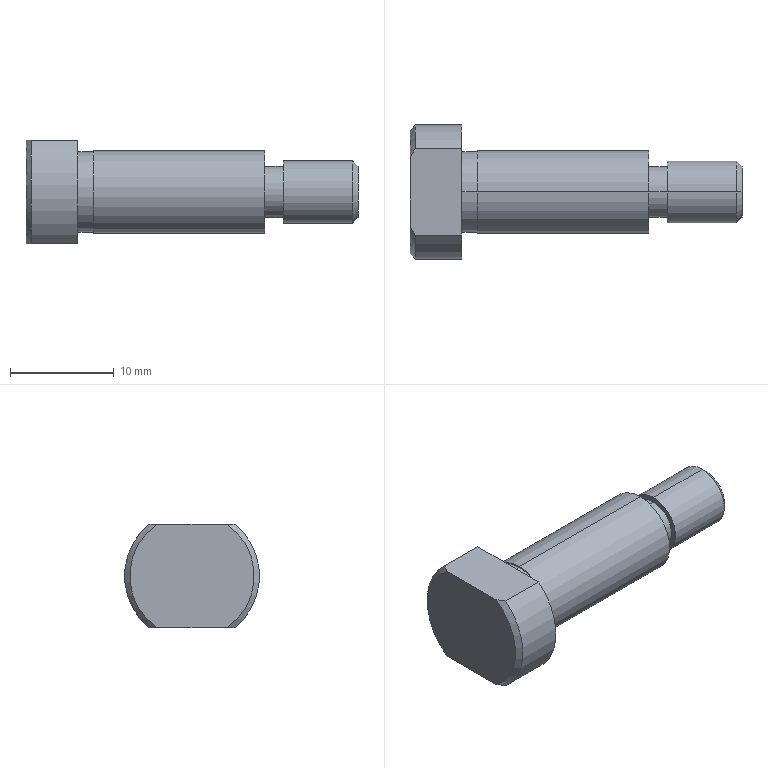Part | STEP file | CLBDG8-18 | 1 solid | 22 faces | box 32 x 13 x 10 mm | volume 1712 mm3 | cylinder 10 | plane 8 | cone 4 | commonest cylinder face diameters 4.917 x2 6 x2 7.8 x2 8 x2 13 x2